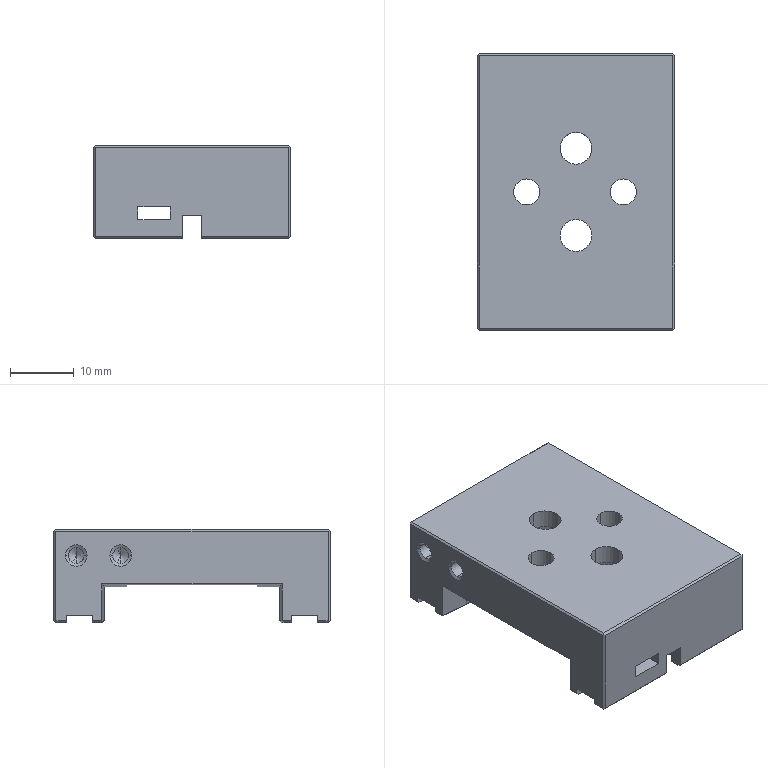Part | NX | 1 solid | 174 faces | box 31 x 43.4 x 14.65 mm | volume 12556 mm3 | plane 85 | cylinder 55 | cone 34 | commonest cylinder face diameters 2.5 x43 4.1 x4 5 x4 9 x4